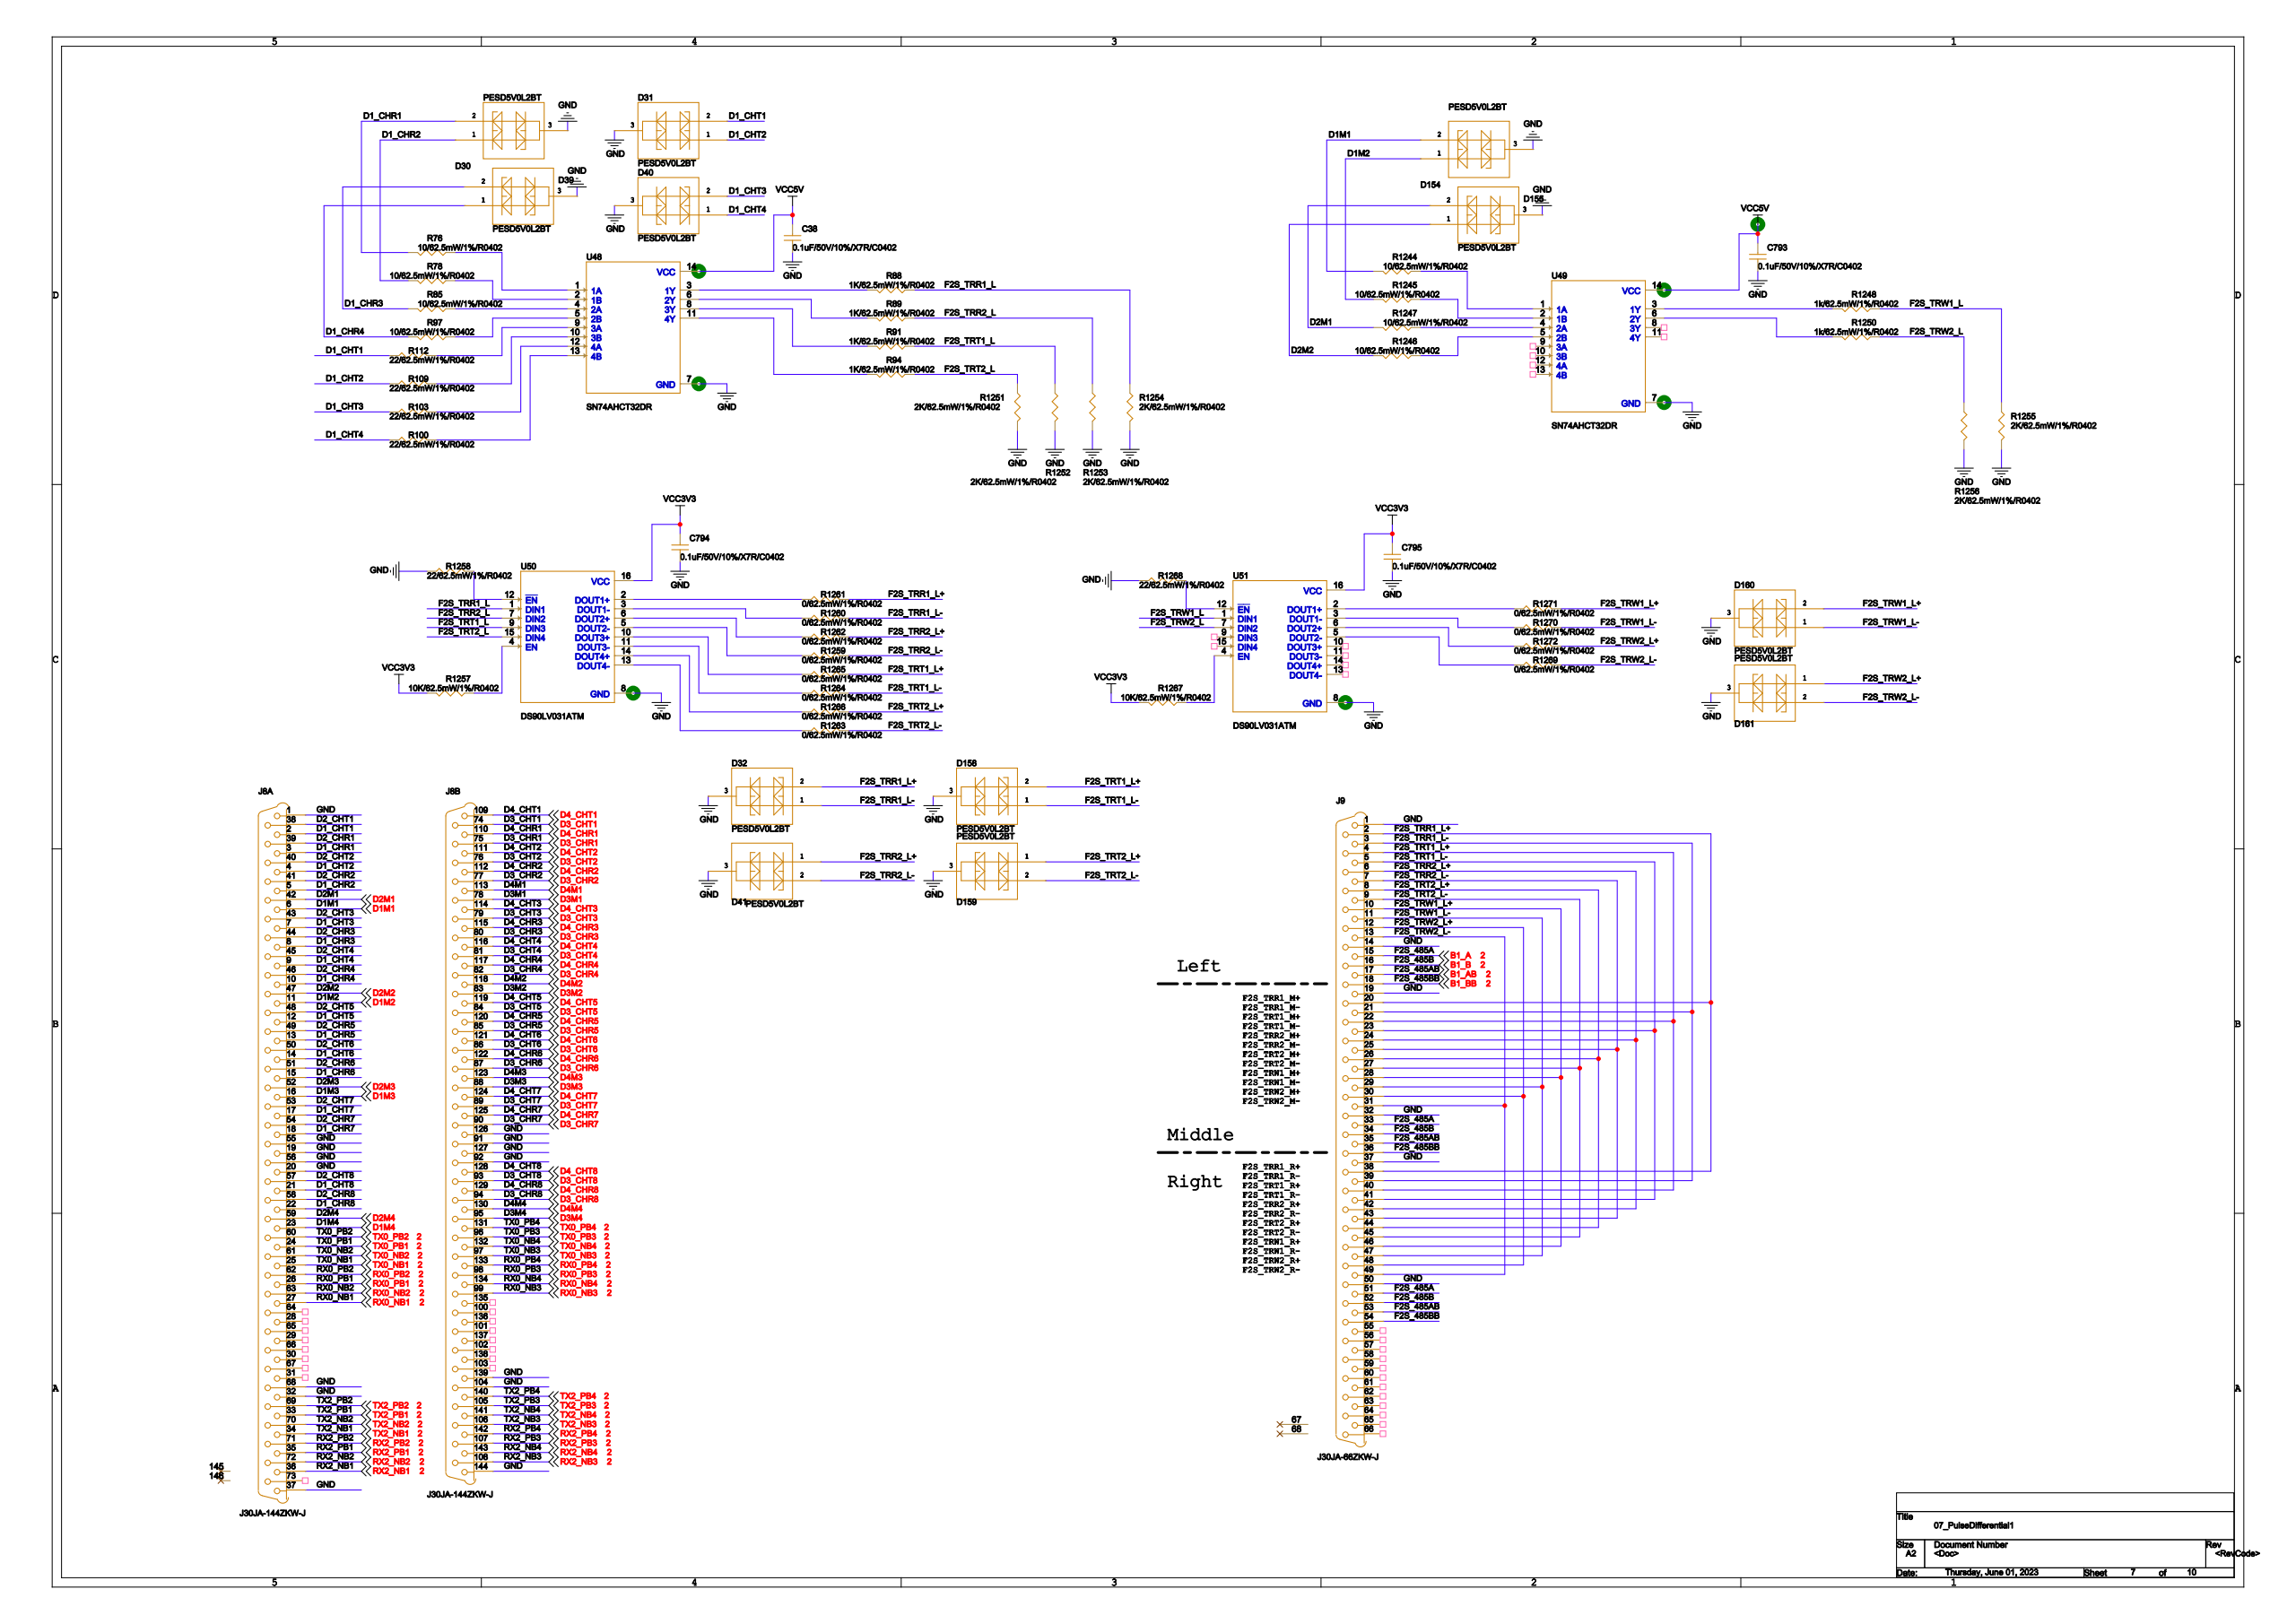Circuit board | Cadence Allegro | 480 parts | 625 nets | one sheet of the schematic
Parts on this sheet (reference | value | footprint):
C38 | 0.1uF/50V/10%/X7R/C0402 | 0402
C793 | 0.1uF/50V/10%/X7R/C0402 | 0402
C794 | 0.1uF/50V/10%/X7R/C0402 | 0402
C795 | 0.1uF/50V/10%/X7R/C0402 | 0402
D30 | PESD5V0L2BT | SOT23
D31 | PESD5V0L2BT | SOT23
D32 | PESD5V0L2BT | SOT23
D39 | PESD5V0L2BT | SOT23
D40 | PESD5V0L2BT | SOT23
D154 | PESD5V0L2BT | SOT23
D155 | PESD5V0L2BT | SOT23
D158 | PESD5V0L2BT | SOT23
D159 | PESD5V0L2BT | SOT23
D160 | PESD5V0L2BT | SOT23
D161 | PESD5V0L2BT | SOT23
J8 | J30JA-144ZKW-J | J30JA-144ZKW-J
J9 | J30JA-66ZKW-J | J30JA-66ZKW-J
R76 | 10/62.5mW/1%/R0402 | 0402
R78 | 10/62.5mW/1%/R0402 | 0402
R85 | 10/62.5mW/1%/R0402 | 0402
R88 | 1k/62.5mW/1%/R0402 | 0402
R89 | 1k/62.5mW/1%/R0402 | 0402
R91 | 1k/62.5mW/1%/R0402 | 0402
R94 | 1k/62.5mW/1%/R0402 | 0402
R97 | 10/62.5mW/1%/R0402 | 0402
R100 | 22/62.5mW/1%/R0402 | 0402
R103 | 22/62.5mW/1%/R0402 | 0402
R109 | 22/62.5mW/1%/R0402 | 0402
R112 | 22/62.5mW/1%/R0402 | 0402
R1244 | 10/62.5mW/1%/R0402 | 0402
R1245 | 10/62.5mW/1%/R0402 | 0402
R1246 | 10/62.5mW/1%/R0402 | 0402
R1247 | 10/62.5mW/1%/R0402 | 0402
R1248 | 1k/62.5mW/1%/R0402 | 0402
R1250 | 1k/62.5mW/1%/R0402 | 0402
R1251 | 2K/62.5mW/1%/R0402 | 0402
R1252 | 2K/62.5mW/1%/R0402 | 0402
R1253 | 2K/62.5mW/1%/R0402 | 0402
R1254 | 2K/62.5mW/1%/R0402 | 0402
R1255 | 2K/62.5mW/1%/R0402 | 0402
R1256 | 2K/62.5mW/1%/R0402 | 0402
R1257 | 10K/62.5mW/1%/R0402 | 0402
R1258 | 22/62.5mW/1%/R0402 | 0402
R1259 | 0/62.5mW/1%/R0402 | 0402
R1260 | 0/62.5mW/1%/R0402 | 0402
R1261 | 0/62.5mW/1%/R0402 | 0402
R1262 | 0/62.5mW/1%/R0402 | 0402
R1263 | 0/62.5mW/1%/R0402 | 0402
R1264 | 0/62.5mW/1%/R0402 | 0402
R1265 | 0/62.5mW/1%/R0402 | 0402
R1266 | 0/62.5mW/1%/R0402 | 0402
R1267 | 10K/62.5mW/1%/R0402 | 0402
R1268 | 22/62.5mW/1%/R0402 | 0402
R1269 | 0/62.5mW/1%/R0402 | 0402
R1270 | 0/62.5mW/1%/R0402 | 0402
R1271 | 0/62.5mW/1%/R0402 | 0402
R1272 | 0/62.5mW/1%/R0402 | 0402
U48 | SN74AHCT32DR | SOIC127P600X175-14N
U49 | SN74AHCT32DR | SOIC127P600X175-14N
U50 | DS90LV031ATM | SOIC127P600X175-16N
U51 | DS90LV031ATM | SOIC127P600X175-16N
Nets of these parts (net: part-pin ...):
AGND: C38-2 C793-2 C794-2 C795-2 D30-3 D31-3 D32-3 D39-3 D40-3 D154-3 D155-3 D158-3 D159-3 D160-3 D161-3 R1251-1 R1252-1 R1253-1 R1254-1 R1255-1 R1256-1 R1258-2 R1268-2 U48-7 U49-7 U50-8 U51-8 J8-1 J8-19 J8-20 J8-32 J8-37 J8-55 J8-56 J8-68 J8-91 J8-92 J8-104 J8-126 J8-127 J8-139 J8-144 J9-1 J9-14 J9-19 J9-32 J9-37 J9-50
3.3V: C794-1 C795-1 R1257-1 R1267-1 U50-16 U51-16
VCC5V: C38-1 C793-1 U48-14 U49-14
N23697083: R1248-1 U49-3
F2S_TRW1_L: R1248-2 R1255-2 U51-1
N23696789: R1250-1 U49-6
F2S_TRW2_L: R1250-2 R1256-2 U51-7
N23232634: R88-1 U48-3
F2S_TRR1_L: R88-2 R1254-2 U50-1
N23696097: R89-1 U48-6
F2S_TRR2_L: R89-2 R1253-2 U50-7
N23232626: R91-1 U48-8
F2S_TRT1_L: R91-2 R1252-2 U50-9
N23232617: R94-1 U48-11
F2S_TRT2_L: R94-2 R1251-2 U50-15
F2S_TRR2_L-: R1259-1 J9-7 J9-25 J9-43
N23702328: R1259-2 U50-5
F2S_TRR1_L-: D32-1 R1260-1 J9-3 J9-21 J9-39
N23702331: R1260-2 U50-3
F2S_TRR1_L+: D32-2 R1261-1 J9-2 J9-20 J9-38
N23702337: R1261-2 U50-2
F2S_TRR2_L+: R1262-1 J9-6 J9-24 J9-42
N23702334: R1262-2 U50-6
F2S_TRT2_L-: D159-2 R1263-1 J9-9 J9-27 J9-45
N23702597: R1263-2 U50-13
F2S_TRT1_L-: D158-1 R1264-1 J9-5 J9-23 J9-41
N23702599: R1264-2 U50-11
F2S_TRT1_L+: D158-2 R1265-1 J9-4 J9-22 J9-40
N23702611: R1265-2 U50-10
F2S_TRT2_L+: D159-1 R1266-1 J9-8 J9-26 J9-44
N23702601: R1266-2 U50-14
F2S_TRW2_L-: D161-2 R1269-1 J9-13 J9-31 J9-49
N23703334: R1269-2 U51-5
F2S_TRW1_L-: D160-1 R1270-1 J9-11 J9-29 J9-47
N23703336: R1270-2 U51-3
F2S_TRW1_L+: D160-2 R1271-1 J9-10 J9-28 J9-46
N23703348: R1271-2 U51-2
F2S_TRW2_L+: D161-1 R1272-1 J9-12 J9-30 J9-48
N23703338: R1272-2 U51-6
B1_A: J9-15 J9-33 J9-51
B1_B: J9-16 J9-34 J9-52
B1_AB: J9-17 J9-35 J9-53
B1_BB: J9-18 J9-36 J9-54
N23232493: R76-2 U48-1
N23232474: R78-2 U48-2
N23232447: R85-2 U48-4
N23232438: R97-2 U48-5
N23695895: R112-1 U48-9
N23695904: R109-1 U48-10
N23695913: R103-1 U48-12
N23695922: R100-1 U48-13
N23697063: R1244-2 U49-1
N23697057: R1245-2 U49-2
N23697050: R1247-2 U49-4
N23697044: R1246-2 U49-5
N23701982: R1257-2 U50-4
N23701987: R1258-1 U50-12
N23703288: R1267-2 U51-4
N23703292: R1268-1 U51-12
D1_CHR4: D39-1 R97-1 J8-10
D1M2: D154-1 R1245-1 J8-11
D1_CHT5: J8-12
D1_CHR5: J8-13
D1_CHT6: J8-14
D1_CHR6: J8-15
D1M3: J8-16
D1_CHT7: J8-17
D1_CHR7: J8-18
D1_CHT1: D31-2 R112-2 J8-2
D1_CHT8: J8-21
D1_CHR8: J8-22
D1M4: J8-23
TX0_PB1: J8-24
TX0_NB1: J8-25
RX0_PB1: J8-26
RX0_NB1: J8-27
D1_CHR1: D30-2 R76-1 J8-3
TX2_PB1: J8-33
TX2_NB1: J8-34
RX2_PB1: J8-35
RX2_NB1: J8-36
D2_CHT1: J8-38
D2_CHR1: J8-39
D1_CHT2: D31-1 R109-2 J8-4
D2_CHT2: J8-40
D2_CHR2: J8-41
D2M1: D155-2 R1247-1 J8-42
D2_CHT3: J8-43
D2_CHR3: J8-44
D2_CHT4: J8-45
D2_CHR4: J8-46
D2M2: D155-1 R1246-1 J8-47
D2_CHT5: J8-48
D2_CHR5: J8-49
D1_CHR2: D30-1 R78-1 J8-5
D2_CHT6: J8-50
D2_CHR6: J8-51
D2M3: J8-52
D2_CHT7: J8-53
D2_CHR7: J8-54
D2_CHT8: J8-57
D2_CHR8: J8-58
D2M4: J8-59
D1M1: D154-2 R1244-1 J8-6
TX0_PB2: J8-60
TX0_NB2: J8-61
RX0_PB2: J8-62
RX0_NB2: J8-63
TX2_PB2: J8-69
D1_CHT3: D40-2 R103-2 J8-7
TX2_NB2: J8-70
RX2_PB2: J8-71
RX2_NB2: J8-72
D1_CHR3: D39-2 R85-1 J8-8
D1_CHT4: D40-1 R100-2 J8-9
TX2_PB3: J8-105
TX2_NB3: J8-106
RX2_PB3: J8-107
RX2_NB3: J8-108
D4_CHT1: J8-109
D4_CHR1: J8-110
D4_CHT2: J8-111
D4_CHR2: J8-112
D4M1: J8-113
D4_CHT3: J8-114
D4_CHR3: J8-115
D4_CHT4: J8-116
D4_CHR4: J8-117
D4M2: J8-118
D4_CHT5: J8-119
D4_CHR5: J8-120
D4_CHT6: J8-121
D4_CHR6: J8-122
D4M3: J8-123
D4_CHT7: J8-124
D4_CHR7: J8-125
D4_CHT8: J8-128
D4_CHR8: J8-129
D4M4: J8-130
TX0_PB4: J8-131
TX0_NB4: J8-132
RX0_PB4: J8-133
RX0_NB4: J8-134
TX2_PB4: J8-140
TX2_NB4: J8-141
RX2_PB4: J8-142
RX2_NB4: J8-143
D3_CHT1: J8-74
D3_CHR1: J8-75
D3_CHT2: J8-76
D3_CHR2: J8-77
D3M1: J8-78
D3_CHT3: J8-79
D3_CHR3: J8-80
D3_CHT4: J8-81
D3_CHR4: J8-82
D3M2: J8-83
D3_CHT5: J8-84
D3_CHR5: J8-85
D3_CHT6: J8-86
D3_CHR6: J8-87
D3M3: J8-88
D3_CHT7: J8-89
D3_CHR7: J8-90
D3_CHT8: J8-93
D3_CHR8: J8-94
D3M4: J8-95
TX0_PB3: J8-96
TX0_NB3: J8-97
RX0_PB3: J8-98
RX0_NB3: J8-99